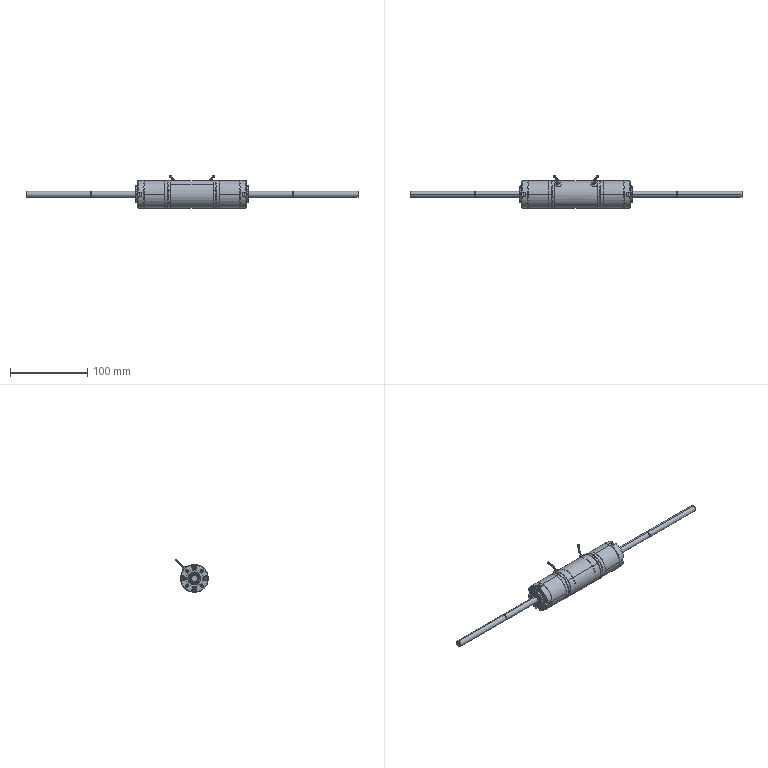Part | SolidWorks | features ReferencePattern 12, MirrorCompFeat 1 | 68 solids | 10898 faces | volume 139903 mm3 | cylinder 4400 | cone 3694 | torus 998 | plane 842 | sphere 680 | spline 284 | commonest cylinder face diameters 1 x1704 3 x1604 24.25 x94 21.991 x92 0.2 x78 1.179 x56